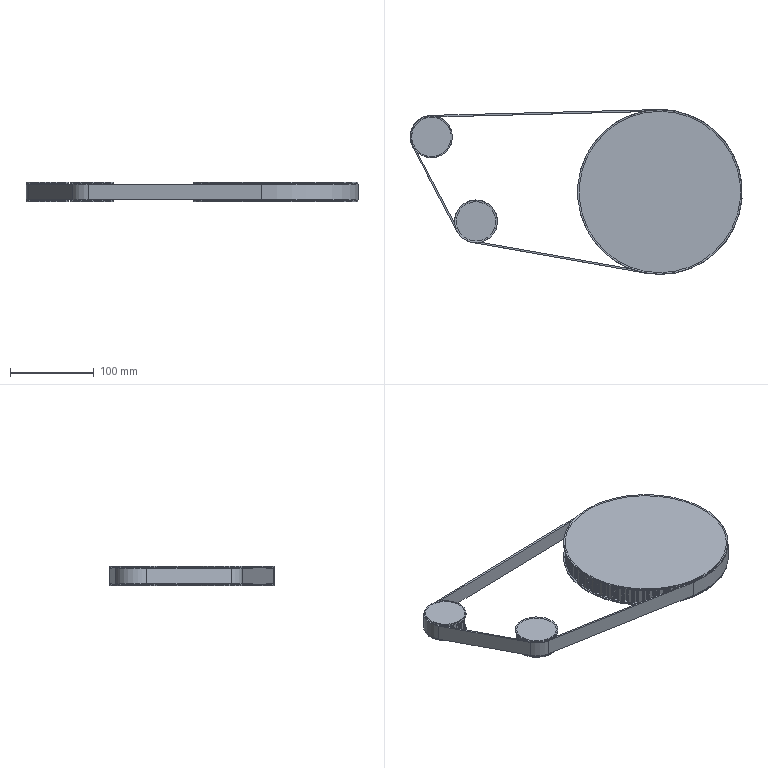Part | SolidWorks | 4 solids | 1078 faces | box 396.622 x 196.734 x 23.437 mm | volume 756376 mm3 | cylinder 656 | plane 374 | cone 36 | torus 12 | commonest cylinder face diameters 3.2 x576 192.67 x50 47.139 x26 51.203 x2 196.734 x2